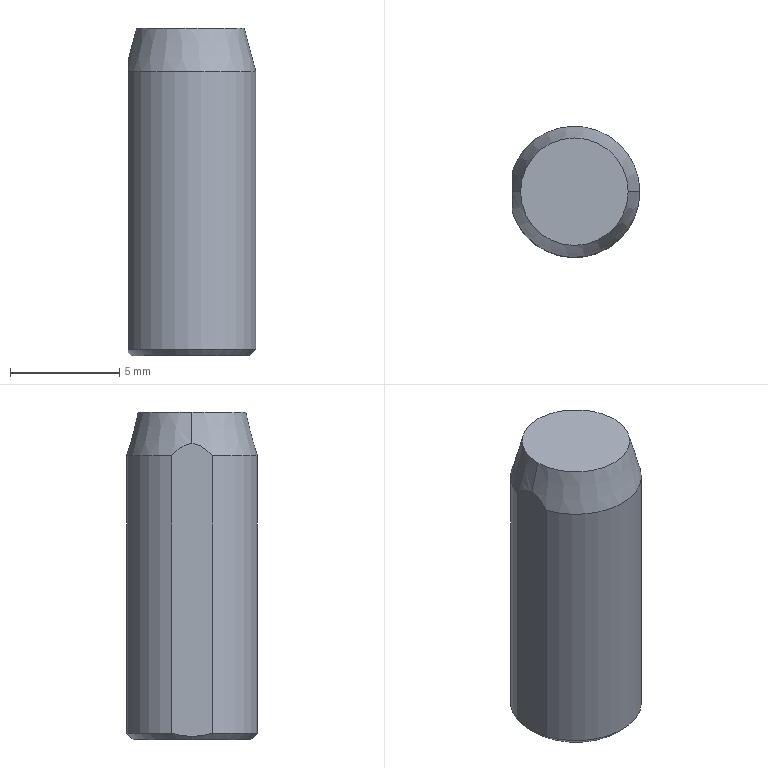Part | STEP file | J454-EBZ05-36-04-Part-1-4 | 1 solid | 14 faces | box 5.854 x 6 x 15 mm | volume 329.867 mm3 | cone 8 | cylinder 3 | plane 3 | commonest cylinder face diameters 3.242 x2 6 x1